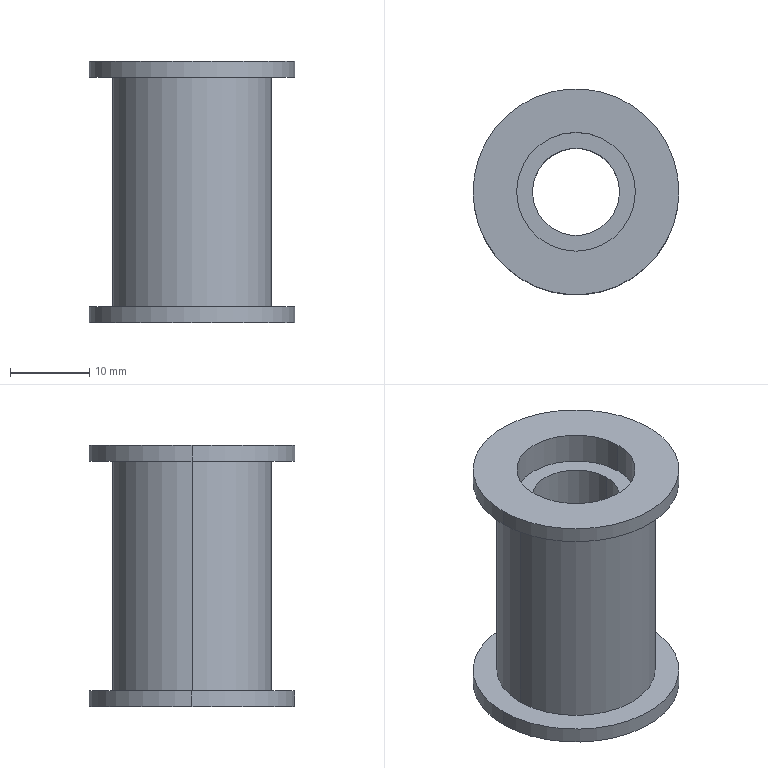Part | STEP file | (PA01.001.LX017) Idler C | 1 solid | 18 faces | box 26 x 26 x 33 mm | volume 7445 mm3 | cylinder 12 | plane 6 | commonest cylinder face diameters 15 x4 26 x4 11 x2 20 x2
STEP:
#1=CARTESIAN_POINT('',(0.,0.,0.));
#2=DIRECTION('',(0.,0.,1.));
#3=DIRECTION('',(1.,0.,0.));
#4=AXIS2_PLACEMENT_3D('',#1,#2,#3);
#5=CARTESIAN_POINT('',(-7.5,0.,-12.5));
#6=VERTEX_POINT('',#5);
#7=CARTESIAN_POINT('',(-7.5,0.,-16.5));
#8=VERTEX_POINT('',#7);
#9=CARTESIAN_POINT('',(-7.5,0.,-12.5));
#10=DIRECTION('',(0.,0.,-1.));
#11=VECTOR('',#10,1.);
#12=LINE('',#9,#11);
#13=CARTESIAN_POINT('',(0.,0.,-12.5));
#14=DIRECTION('',(0.,0.,-1.));
#15=DIRECTION('',(-1.,0.,0.));
#16=AXIS2_PLACEMENT_3D('',#13,#14,#15);
#17=CYLINDRICAL_SURFACE('',#16,7.5);
#18=CARTESIAN_POINT('',(6.283,0.));
#19=DIRECTION('',(0.,1.));
#20=VECTOR('',#19,1.);
#21=LINE('',#18,#20);
#22=(GEOMETRIC_REPRESENTATION_CONTEXT(2)PARAMETRIC_REPRESENTATION_CONTEXT()REPRESENTATION_CONTEXT('',''));
#23=DEFINITIONAL_REPRESENTATION('',(#21),#22);
#24=PCURVE('',#17,#23);
#25=CARTESIAN_POINT('',(0.,0.,-12.5));
#26=DIRECTION('',(0.,0.,-1.));
#27=DIRECTION('',(-1.,0.,0.));
#28=AXIS2_PLACEMENT_3D('',#25,#26,#27);
#29=CYLINDRICAL_SURFACE('',#28,7.5);
#30=CARTESIAN_POINT('',(0.,0.));
#31=DIRECTION('',(0.,1.));
#32=VECTOR('',#31,1.);
#33=LINE('',#30,#32);
#34=(GEOMETRIC_REPRESENTATION_CONTEXT(2)PARAMETRIC_REPRESENTATION_CONTEXT()REPRESENTATION_CONTEXT('',''));
#35=DEFINITIONAL_REPRESENTATION('',(#33),#34);
#36=PCURVE('',#29,#35);
#37=SURFACE_CURVE('',#12,(#24,#36),.PCURVE_S1.);
#38=EDGE_CURVE('',#6,#8,#37,.T.);
#39=ORIENTED_EDGE('',*,*,#38,.T.);
#40=CARTESIAN_POINT('',(7.5,0.,-16.5));
#41=VERTEX_POINT('',#40);
#42=CARTESIAN_POINT('',(0.,0.,-16.5));
#43=DIRECTION('',(0.,0.,-1.));
#44=DIRECTION('',(-1.,0.,0.));
#45=AXIS2_PLACEMENT_3D('',#42,#43,#44);
#46=CIRCLE('',#45,7.5);
#47=CARTESIAN_POINT('',(0.,4.));
#48=DIRECTION('',(1.,0.));
#49=VECTOR('',#48,1.);
#50=LINE('',#47,#49);
#51=(GEOMETRIC_REPRESENTATION_CONTEXT(2)PARAMETRIC_REPRESENTATION_CONTEXT()REPRESENTATION_CONTEXT('',''));
#52=DEFINITIONAL_REPRESENTATION('',(#50),#51);
#53=PCURVE('',#17,#52);
#54=CARTESIAN_POINT('',(0.,0.,-16.5));
#55=DIRECTION('',(0.,0.,-1.));
#56=DIRECTION('',(-1.,0.,0.));
#57=AXIS2_PLACEMENT_3D('',#54,#55,#56);
#58=PLANE('',#57);
#59=CARTESIAN_POINT('',(0.,0.));
#60=DIRECTION('',(1.,0.));
#61=AXIS2_PLACEMENT_2D('',#59,#60);
#62=CIRCLE('',#61,7.5);
#63=(GEOMETRIC_REPRESENTATION_CONTEXT(2)PARAMETRIC_REPRESENTATION_CONTEXT()REPRESENTATION_CONTEXT('',''));
#64=DEFINITIONAL_REPRESENTATION('',(#62),#63);
#65=PCURVE('',#58,#64);
#66=SURFACE_CURVE('',#46,(#53,#65),.PCURVE_S1.);
#67=EDGE_CURVE('',#41,#8,#66,.T.);
#68=ORIENTED_EDGE('',*,*,#67,.F.);
#69=CARTESIAN_POINT('',(7.5,0.,-12.5));
#70=VERTEX_POINT('',#69);
#71=CARTESIAN_POINT('',(7.5,0.,-12.5));
#72=DIRECTION('',(0.,0.,-1.));
#73=VECTOR('',#72,1.);
#74=LINE('',#71,#73);
#75=CARTESIAN_POINT('',(3.142,0.));
#76=DIRECTION('',(0.,1.));
#77=VECTOR('',#76,1.);
#78=LINE('',#75,#77);
#79=(GEOMETRIC_REPRESENTATION_CONTEXT(2)PARAMETRIC_REPRESENTATION_CONTEXT()REPRESENTATION_CONTEXT('',''));
#80=DEFINITIONAL_REPRESENTATION('',(#78),#79);
#81=PCURVE('',#17,#80);
#82=CARTESIAN_POINT('',(3.142,0.));
#83=DIRECTION('',(0.,1.));
#84=VECTOR('',#83,1.);
#85=LINE('',#82,#84);
#86=(GEOMETRIC_REPRESENTATION_CONTEXT(2)PARAMETRIC_REPRESENTATION_CONTEXT()REPRESENTATION_CONTEXT('',''));
#87=DEFINITIONAL_REPRESENTATION('',(#85),#86);
#88=PCURVE('',#29,#87);
#89=SURFACE_CURVE('',#74,(#81,#88),.PCURVE_S1.);
#90=EDGE_CURVE('',#70,#41,#89,.T.);
#91=ORIENTED_EDGE('',*,*,#90,.F.);
#92=CARTESIAN_POINT('',(0.,0.,-12.5));
#93=DIRECTION('',(0.,0.,-1.));
#94=DIRECTION('',(-1.,0.,0.));
#95=AXIS2_PLACEMENT_3D('',#92,#93,#94);
#96=CIRCLE('',#95,7.5);
#97=CARTESIAN_POINT('',(0.,0.));
#98=DIRECTION('',(1.,0.));
#99=VECTOR('',#98,1.);
#100=LINE('',#97,#99);
#101=(GEOMETRIC_REPRESENTATION_CONTEXT(2)PARAMETRIC_REPRESENTATION_CONTEXT()REPRESENTATION_CONTEXT('',''));
#102=DEFINITIONAL_REPRESENTATION('',(#100),#101);
#103=PCURVE('',#17,#102);
#104=CARTESIAN_POINT('',(0.,0.,-12.5));
#105=DIRECTION('',(0.,0.,-1.));
#106=DIRECTION('',(-1.,0.,0.));
#107=AXIS2_PLACEMENT_3D('',#104,#105,#106);
#108=PLANE('',#107);
#109=CARTESIAN_POINT('',(0.,0.));
#110=DIRECTION('',(1.,0.));
#111=AXIS2_PLACEMENT_2D('',#109,#110);
#112=CIRCLE('',#111,7.5);
#113=(GEOMETRIC_REPRESENTATION_CONTEXT(2)PARAMETRIC_REPRESENTATION_CONTEXT()REPRESENTATION_CONTEXT('',''));
#114=DEFINITIONAL_REPRESENTATION('',(#112),#113);
#115=PCURVE('',#108,#114);
#116=SURFACE_CURVE('',#96,(#103,#115),.PCURVE_S1.);
#117=EDGE_CURVE('',#70,#6,#116,.T.);
#118=ORIENTED_EDGE('',*,*,#117,.T.);
#119=EDGE_LOOP('',(#39,#68,#91,#118));
#120=FACE_BOUND('',#119,.F.);
#121=ADVANCED_FACE('',(#120),#17,.F.);
#122=CARTESIAN_POINT('',(7.5,0.,12.5));
#123=VERTEX_POINT('',#122);
#124=CARTESIAN_POINT('',(7.5,0.,16.5));
#125=VERTEX_POINT('',#124);
#126=CARTESIAN_POINT('',(7.5,0.,12.5));
#127=DIRECTION('',(0.,0.,1.));
#128=VECTOR('',#127,1.);
#129=LINE('',#126,#128);
#130=CARTESIAN_POINT('',(0.,0.,12.5));
#131=DIRECTION('',(0.,0.,1.));
#132=DIRECTION('',(1.,0.,0.));
#133=AXIS2_PLACEMENT_3D('',#130,#131,#132);
#134=CYLINDRICAL_SURFACE('',#133,7.5);
#135=CARTESIAN_POINT('',(6.283,0.));
#136=DIRECTION('',(0.,1.));
#137=VECTOR('',#136,1.);
#138=LINE('',#135,#137);
#139=(GEOMETRIC_REPRESENTATION_CONTEXT(2)PARAMETRIC_REPRESENTATION_CONTEXT()REPRESENTATION_CONTEXT('',''));
#140=DEFINITIONAL_REPRESENTATION('',(#138),#139);
#141=PCURVE('',#134,#140);
#142=CARTESIAN_POINT('',(0.,0.,12.5));
#143=DIRECTION('',(0.,0.,1.));
#144=DIRECTION('',(1.,0.,0.));
#145=AXIS2_PLACEMENT_3D('',#142,#143,#144);
#146=CYLINDRICAL_SURFACE('',#145,7.5);
#147=CARTESIAN_POINT('',(0.,0.));
#148=DIRECTION('',(0.,1.));
#149=VECTOR('',#148,1.);
#150=LINE('',#147,#149);
#151=(GEOMETRIC_REPRESENTATION_CONTEXT(2)PARAMETRIC_REPRESENTATION_CONTEXT()REPRESENTATION_CONTEXT('',''));
#152=DEFINITIONAL_REPRESENTATION('',(#150),#151);
#153=PCURVE('',#146,#152);
#154=SURFACE_CURVE('',#129,(#141,#153),.PCURVE_S1.);
#155=EDGE_CURVE('',#123,#125,#154,.T.);
#156=ORIENTED_EDGE('',*,*,#155,.T.);
#157=CARTESIAN_POINT('',(-7.5,0.,16.5));
#158=VERTEX_POINT('',#157);
#159=CARTESIAN_POINT('',(0.,0.,16.5));
#160=DIRECTION('',(0.,0.,1.));
#161=DIRECTION('',(1.,0.,0.));
#162=AXIS2_PLACEMENT_3D('',#159,#160,#161);
#163=CIRCLE('',#162,7.5);
#164=CARTESIAN_POINT('',(0.,4.));
#165=DIRECTION('',(1.,0.));
#166=VECTOR('',#165,1.);
#167=LINE('',#164,#166);
#168=(GEOMETRIC_REPRESENTATION_CONTEXT(2)PARAMETRIC_REPRESENTATION_CONTEXT()REPRESENTATION_CONTEXT('',''));
#169=DEFINITIONAL_REPRESENTATION('',(#167),#168);
#170=PCURVE('',#134,#169);
#171=CARTESIAN_POINT('',(0.,0.,16.5));
#172=DIRECTION('',(0.,0.,1.));
#173=DIRECTION('',(1.,0.,0.));
#174=AXIS2_PLACEMENT_3D('',#171,#172,#173);
#175=PLANE('',#174);
#176=CARTESIAN_POINT('',(0.,0.));
#177=DIRECTION('',(1.,0.));
#178=AXIS2_PLACEMENT_2D('',#176,#177);
#179=CIRCLE('',#178,7.5);
#180=(GEOMETRIC_REPRESENTATION_CONTEXT(2)PARAMETRIC_REPRESENTATION_CONTEXT()REPRESENTATION_CONTEXT('',''));
#181=DEFINITIONAL_REPRESENTATION('',(#179),#180);
#182=PCURVE('',#175,#181);
#183=SURFACE_CURVE('',#163,(#170,#182),.PCURVE_S1.);
#184=EDGE_CURVE('',#158,#125,#183,.T.);
#185=ORIENTED_EDGE('',*,*,#184,.F.);
#186=CARTESIAN_POINT('',(-7.5,0.,12.5));
#187=VERTEX_POINT('',#186);
#188=CARTESIAN_POINT('',(-7.5,0.,12.5));
#189=DIRECTION('',(0.,0.,1.));
#190=VECTOR('',#189,1.);
#191=LINE('',#188,#190);
#192=CARTESIAN_POINT('',(3.142,0.));
#193=DIRECTION('',(0.,1.));
#194=VECTOR('',#193,1.);
#195=LINE('',#192,#194);
#196=(GEOMETRIC_REPRESENTATION_CONTEXT(2)PARAMETRIC_REPRESENTATION_CONTEXT()REPRESENTATION_CONTEXT('',''));
#197=DEFINITIONAL_REPRESENTATION('',(#195),#196);
#198=PCURVE('',#134,#197);
#199=CARTESIAN_POINT('',(3.142,0.));
#200=DIRECTION('',(0.,1.));
#201=VECTOR('',#200,1.);
#202=LINE('',#199,#201);
#203=(GEOMETRIC_REPRESENTATION_CONTEXT(2)PARAMETRIC_REPRESENTATION_CONTEXT()REPRESENTATION_CONTEXT('',''));
#204=DEFINITIONAL_REPRESENTATION('',(#202),#203);
#205=PCURVE('',#146,#204);
#206=SURFACE_CURVE('',#191,(#198,#205),.PCURVE_S1.);
#207=EDGE_CURVE('',#187,#158,#206,.T.);
#208=ORIENTED_EDGE('',*,*,#207,.F.);
#209=CARTESIAN_POINT('',(0.,0.,12.5));
#210=DIRECTION('',(0.,0.,1.));
#211=DIRECTION('',(1.,0.,0.));
#212=AXIS2_PLACEMENT_3D('',#209,#210,#211);
#213=CIRCLE('',#212,7.5);
#214=CARTESIAN_POINT('',(0.,0.));
#215=DIRECTION('',(1.,0.));
#216=VECTOR('',#215,1.);
#217=LINE('',#214,#216);
#218=(GEOMETRIC_REPRESENTATION_CONTEXT(2)PARAMETRIC_REPRESENTATION_CONTEXT()REPRESENTATION_CONTEXT('',''));
#219=DEFINITIONAL_REPRESENTATION('',(#217),#218);
#220=PCURVE('',#134,#219);
#221=CARTESIAN_POINT('',(0.,0.,12.5));
#222=DIRECTION('',(0.,0.,1.));
#223=DIRECTION('',(1.,0.,0.));
#224=AXIS2_PLACEMENT_3D('',#221,#222,#223);
#225=PLANE('',#224);
#226=CARTESIAN_POINT('',(0.,0.));
#227=DIRECTION('',(1.,0.));
#228=AXIS2_PLACEMENT_2D('',#226,#227);
#229=CIRCLE('',#228,7.5);
#230=(GEOMETRIC_REPRESENTATION_CONTEXT(2)PARAMETRIC_REPRESENTATION_CONTEXT()REPRESENTATION_CONTEXT('',''));
#231=DEFINITIONAL_REPRESENTATION('',(#229),#230);
#232=PCURVE('',#225,#231);
#233=SURFACE_CURVE('',#213,(#220,#232),.PCURVE_S1.);
#234=EDGE_CURVE('',#187,#123,#233,.T.);
#235=ORIENTED_EDGE('',*,*,#234,.T.);
#236=EDGE_LOOP('',(#156,#185,#208,#235));
#237=FACE_BOUND('',#236,.F.);
#238=ADVANCED_FACE('',(#237),#134,.F.);
#239=CARTESIAN_POINT('',(-13.,0.,-16.5));
#240=VERTEX_POINT('',#239);
#241=CARTESIAN_POINT('',(13.,0.,-16.5));
#242=VERTEX_POINT('',#241);
#243=CARTESIAN_POINT('',(0.,0.,-16.5));
#244=DIRECTION('',(0.,0.,-1.));
#245=DIRECTION('',(-1.,0.,0.));
#246=AXIS2_PLACEMENT_3D('',#243,#244,#245);
#247=CIRCLE('',#246,13.);
#248=CARTESIAN_POINT('',(0.,0.,-16.5));
#249=DIRECTION('',(0.,0.,1.));
#250=DIRECTION('',(1.,0.,0.));
#251=AXIS2_PLACEMENT_3D('',#248,#249,#250);
#252=CYLINDRICAL_SURFACE('',#251,13.);
#253=CARTESIAN_POINT('',(3.142,0.));
#254=DIRECTION('',(-1.,0.));
#255=VECTOR('',#254,1.);
#256=LINE('',#253,#255);
#257=(GEOMETRIC_REPRESENTATION_CONTEXT(2)PARAMETRIC_REPRESENTATION_CONTEXT()REPRESENTATION_CONTEXT('',''));
#258=DEFINITIONAL_REPRESENTATION('',(#256),#257);
#259=PCURVE('',#252,#258);
#260=CARTESIAN_POINT('',(0.,0.));
#261=DIRECTION('',(1.,0.));
#262=AXIS2_PLACEMENT_2D('',#260,#261);
#263=CIRCLE('',#262,13.);
#264=(GEOMETRIC_REPRESENTATION_CONTEXT(2)PARAMETRIC_REPRESENTATION_CONTEXT()REPRESENTATION_CONTEXT('',''));
#265=DEFINITIONAL_REPRESENTATION('',(#263),#264);
#266=PCURVE('',#58,#265);
#267=SURFACE_CURVE('',#247,(#259,#266),.PCURVE_S1.);
#268=EDGE_CURVE('',#240,#242,#267,.T.);
#269=ORIENTED_EDGE('',*,*,#268,.F.);
#270=CARTESIAN_POINT('',(-13.,0.,-14.5));
#271=VERTEX_POINT('',#270);
#272=CARTESIAN_POINT('',(-13.,0.,-16.5));
#273=DIRECTION('',(0.,0.,1.));
#274=VECTOR('',#273,1.);
#275=LINE('',#272,#274);
#276=CARTESIAN_POINT('',(3.142,0.));
#277=DIRECTION('',(0.,1.));
#278=VECTOR('',#277,1.);
#279=LINE('',#276,#278);
#280=(GEOMETRIC_REPRESENTATION_CONTEXT(2)PARAMETRIC_REPRESENTATION_CONTEXT()REPRESENTATION_CONTEXT('',''));
#281=DEFINITIONAL_REPRESENTATION('',(#279),#280);
#282=PCURVE('',#252,#281);
#283=CARTESIAN_POINT('',(0.,0.,-16.5));
#284=DIRECTION('',(0.,0.,1.));
#285=DIRECTION('',(1.,0.,0.));
#286=AXIS2_PLACEMENT_3D('',#283,#284,#285);
#287=CYLINDRICAL_SURFACE('',#286,13.);
#288=CARTESIAN_POINT('',(3.142,0.));
#289=DIRECTION('',(0.,1.));
#290=VECTOR('',#289,1.);
#291=LINE('',#288,#290);
#292=(GEOMETRIC_REPRESENTATION_CONTEXT(2)PARAMETRIC_REPRESENTATION_CONTEXT()REPRESENTATION_CONTEXT('',''));
#293=DEFINITIONAL_REPRESENTATION('',(#291),#292);
#294=PCURVE('',#287,#293);
#295=SURFACE_CURVE('',#275,(#282,#294),.PCURVE_S1.);
#296=EDGE_CURVE('',#240,#271,#295,.T.);
#297=ORIENTED_EDGE('',*,*,#296,.T.);
#298=CARTESIAN_POINT('',(13.,0.,-14.5));
#299=VERTEX_POINT('',#298);
#300=CARTESIAN_POINT('',(0.,0.,-14.5));
#301=DIRECTION('',(0.,0.,-1.));
#302=DIRECTION('',(-1.,0.,0.));
#303=AXIS2_PLACEMENT_3D('',#300,#301,#302);
#304=CIRCLE('',#303,13.);
#305=CARTESIAN_POINT('',(3.142,2.));
#306=DIRECTION('',(-1.,0.));
#307=VECTOR('',#306,1.);
#308=LINE('',#305,#307);
#309=(GEOMETRIC_REPRESENTATION_CONTEXT(2)PARAMETRIC_REPRESENTATION_CONTEXT()REPRESENTATION_CONTEXT('',''));
#310=DEFINITIONAL_REPRESENTATION('',(#308),#309);
#311=PCURVE('',#252,#310);
#312=CARTESIAN_POINT('',(0.,0.,-14.5));
#313=DIRECTION('',(0.,0.,-1.));
#314=DIRECTION('',(-1.,0.,0.));
#315=AXIS2_PLACEMENT_3D('',#312,#313,#314);
#316=PLANE('',#315);
#317=CARTESIAN_POINT('',(0.,0.));
#318=DIRECTION('',(1.,0.));
#319=AXIS2_PLACEMENT_2D('',#317,#318);
#320=CIRCLE('',#319,13.);
#321=(GEOMETRIC_REPRESENTATION_CONTEXT(2)PARAMETRIC_REPRESENTATION_CONTEXT()REPRESENTATION_CONTEXT('',''));
#322=DEFINITIONAL_REPRESENTATION('',(#320),#321);
#323=PCURVE('',#316,#322);
#324=SURFACE_CURVE('',#304,(#311,#323),.PCURVE_S1.);
#325=EDGE_CURVE('',#271,#299,#324,.T.);
#326=ORIENTED_EDGE('',*,*,#325,.T.);
#327=CARTESIAN_POINT('',(13.,0.,-16.5));
#328=DIRECTION('',(0.,0.,1.));
#329=VECTOR('',#328,1.);
#330=LINE('',#327,#329);
#331=CARTESIAN_POINT('',(0.,0.));
#332=DIRECTION('',(0.,1.));
#333=VECTOR('',#332,1.);
#334=LINE('',#331,#333);
#335=(GEOMETRIC_REPRESENTATION_CONTEXT(2)PARAMETRIC_REPRESENTATION_CONTEXT()REPRESENTATION_CONTEXT('',''));
#336=DEFINITIONAL_REPRESENTATION('',(#334),#335);
#337=PCURVE('',#252,#336);
#338=CARTESIAN_POINT('',(6.283,0.));
#339=DIRECTION('',(0.,1.));
#340=VECTOR('',#339,1.);
#341=LINE('',#338,#340);
#342=(GEOMETRIC_REPRESENTATION_CONTEXT(2)PARAMETRIC_REPRESENTATION_CONTEXT()REPRESENTATION_CONTEXT('',''));
#343=DEFINITIONAL_REPRESENTATION('',(#341),#342);
#344=PCURVE('',#287,#343);
#345=SURFACE_CURVE('',#330,(#337,#344),.PCURVE_S1.);
#346=EDGE_CURVE('',#242,#299,#345,.T.);
#347=ORIENTED_EDGE('',*,*,#346,.F.);
#348=EDGE_LOOP('',(#269,#297,#326,#347));
#349=FACE_BOUND('',#348,.T.);
#350=ADVANCED_FACE('',(#349),#252,.T.);
#351=CARTESIAN_POINT('',(13.,0.,16.5));
#352=VERTEX_POINT('',#351);
#353=CARTESIAN_POINT('',(-13.,0.,16.5));
#354=VERTEX_POINT('',#353);
#355=CARTESIAN_POINT('',(0.,0.,16.5));
#356=DIRECTION('',(0.,0.,1.));
#357=DIRECTION('',(1.,0.,0.));
#358=AXIS2_PLACEMENT_3D('',#355,#356,#357);
#359=CIRCLE('',#358,13.);
#360=CARTESIAN_POINT('',(0.,0.,16.5));
#361=DIRECTION('',(0.,0.,-1.));
#362=DIRECTION('',(-1.,0.,0.));
#363=AXIS2_PLACEMENT_3D('',#360,#361,#362);
#364=CYLINDRICAL_SURFACE('',#363,13.);
#365=CARTESIAN_POINT('',(3.142,0.));
#366=DIRECTION('',(-1.,0.));
#367=VECTOR('',#366,1.);
#368=LINE('',#365,#367);
#369=(GEOMETRIC_REPRESENTATION_CONTEXT(2)PARAMETRIC_REPRESENTATION_CONTEXT()REPRESENTATION_CONTEXT('',''));
#370=DEFINITIONAL_REPRESENTATION('',(#368),#369);
#371=PCURVE('',#364,#370);
#372=CARTESIAN_POINT('',(0.,0.));
#373=DIRECTION('',(1.,0.));
#374=AXIS2_PLACEMENT_2D('',#372,#373);
#375=CIRCLE('',#374,13.);
#376=(GEOMETRIC_REPRESENTATION_CONTEXT(2)PARAMETRIC_REPRESENTATION_CONTEXT()REPRESENTATION_CONTEXT('',''));
#377=DEFINITIONAL_REPRESENTATION('',(#375),#376);
#378=PCURVE('',#175,#377);
#379=SURFACE_CURVE('',#359,(#371,#378),.PCURVE_S1.);
#380=EDGE_CURVE('',#352,#354,#379,.T.);
#381=ORIENTED_EDGE('',*,*,#380,.F.);
#382=CARTESIAN_POINT('',(13.,0.,14.5));
#383=VERTEX_POINT('',#382);
#384=CARTESIAN_POINT('',(13.,0.,16.5));
#385=DIRECTION('',(0.,0.,-1.));
#386=VECTOR('',#385,1.);
#387=LINE('',#384,#386);
#388=CARTESIAN_POINT('',(3.142,0.));
#389=DIRECTION('',(0.,1.));
#390=VECTOR('',#389,1.);
#391=LINE('',#388,#390);
#392=(GEOMETRIC_REPRESENTATION_CONTEXT(2)PARAMETRIC_REPRESENTATION_CONTEXT()REPRESENTATION_CONTEXT('',''));
#393=DEFINITIONAL_REPRESENTATION('',(#391),#392);
#394=PCURVE('',#364,#393);
#395=CARTESIAN_POINT('',(0.,0.,16.5));
#396=DIRECTION('',(0.,0.,-1.));
#397=DIRECTION('',(-1.,0.,0.));
#398=AXIS2_PLACEMENT_3D('',#395,#396,#397);
#399=CYLINDRICAL_SURFACE('',#398,13.);
#400=CARTESIAN_POINT('',(3.142,0.));
#401=DIRECTION('',(0.,1.));
#402=VECTOR('',#401,1.);
#403=LINE('',#400,#402);
#404=(GEOMETRIC_REPRESENTATION_CONTEXT(2)PARAMETRIC_REPRESENTATION_CONTEXT()REPRESENTATION_CONTEXT('',''));
#405=DEFINITIONAL_REPRESENTATION('',(#403),#404);
#406=PCURVE('',#399,#405);
#407=SURFACE_CURVE('',#387,(#394,#406),.PCURVE_S1.);
#408=EDGE_CURVE('',#352,#383,#407,.T.);
#409=ORIENTED_EDGE('',*,*,#408,.T.);
#410=CARTESIAN_POINT('',(-13.,0.,14.5));
#411=VERTEX_POINT('',#410);
#412=CARTESIAN_POINT('',(0.,0.,14.5));
#413=DIRECTION('',(0.,0.,1.));
#414=DIRECTION('',(1.,0.,0.));
#415=AXIS2_PLACEMENT_3D('',#412,#413,#414);
#416=CIRCLE('',#415,13.);
#417=CARTESIAN_POINT('',(3.142,2.));
#418=DIRECTION('',(-1.,0.));
#419=VECTOR('',#418,1.);
#420=LINE('',#417,#419);
#421=(GEOMETRIC_REPRESENTATION_CONTEXT(2)PARAMETRIC_REPRESENTATION_CONTEXT()REPRESENTATION_CONTEXT('',''));
#422=DEFINITIONAL_REPRESENTATION('',(#420),#421);
#423=PCURVE('',#364,#422);
#424=CARTESIAN_POINT('',(0.,0.,14.5));
#425=DIRECTION('',(0.,0.,1.));
#426=DIRECTION('',(1.,0.,0.));
#427=AXIS2_PLACEMENT_3D('',#424,#425,#426);
#428=PLANE('',#427);
#429=CARTESIAN_POINT('',(0.,0.));
#430=DIRECTION('',(1.,0.));
#431=AXIS2_PLACEMENT_2D('',#429,#430);
#432=CIRCLE('',#431,13.);
#433=(GEOMETRIC_REPRESENTATION_CONTEXT(2)PARAMETRIC_REPRESENTATION_CONTEXT()REPRESENTATION_CONTEXT('',''));
#434=DEFINITIONAL_REPRESENTATION('',(#432),#433);
#435=PCURVE('',#428,#434);
#436=SURFACE_CURVE('',#416,(#423,#435),.PCURVE_S1.);
#437=EDGE_CURVE('',#383,#411,#436,.T.);
#438=ORIENTED_EDGE('',*,*,#437,.T.);
#439=CARTESIAN_POINT('',(-13.,0.,16.5));
#440=DIRECTION('',(0.,0.,-1.));
#441=VECTOR('',#440,1.);
#442=LINE('',#439,#441);
#443=CARTESIAN_POINT('',(0.,0.));
#444=DIRECTION('',(0.,1.));
#445=VECTOR('',#444,1.);
#446=LINE('',#443,#445);
#447=(GEOMETRIC_REPRESENTATION_CONTEXT(2)PARAMETRIC_REPRESENTATION_CONTEXT()REPRESENTATION_CONTEXT('',''));
#448=DEFINITIONAL_REPRESENTATION('',(#446),#447);
#449=PCURVE('',#364,#448);
#450=CARTESIAN_POINT('',(6.283,0.));
#451=DIRECTION('',(0.,1.));
#452=VECTOR('',#451,1.);
#453=LINE('',#450,#452);
#454=(GEOMETRIC_REPRESENTATION_CONTEXT(2)PARAMETRIC_REPRESENTATION_CONTEXT()REPRESENTATION_CONTEXT('',''));
#455=DEFINITIONAL_REPRESENTATION('',(#453),#454);
#456=PCURVE('',#399,#455);
#457=SURFACE_CURVE('',#442,(#449,#456),.PCURVE_S1.);
#458=EDGE_CURVE('',#354,#411,#457,.T.);
#459=ORIENTED_EDGE('',*,*,#458,.F.);
#460=EDGE_LOOP('',(#381,#409,#438,#459));
#461=FACE_BOUND('',#460,.T.);
#462=ADVANCED_FACE('',(#461),#364,.T.);
#463=CARTESIAN_POINT('',(10.,0.,14.5));
#464=VERTEX_POINT('',#463);
#465=CARTESIAN_POINT('',(-10.,0.,14.5));
#466=VERTEX_POINT('',#465);
#467=CARTESIAN_POINT('',(0.,0.,14.5));
#468=DIRECTION('',(0.,0.,1.));
#469=DIRECTION('',(1.,0.,0.));
#470=AXIS2_PLACEMENT_3D('',#467,#468,#469);
#471=CIRCLE('',#470,10.);
#472=CARTESIAN_POINT('',(0.,0.,14.5));
#473=DIRECTION('',(0.,0.,-1.));
#474=DIRECTION('',(-1.,0.,0.));
#475=AXIS2_PLACEMENT_3D('',#472,#473,#474);
#476=CYLINDRICAL_SURFACE('',#475,10.);
#477=CARTESIAN_POINT('',(3.142,0.));
#478=DIRECTION('',(-1.,0.));
#479=VECTOR('',#478,1.);
#480=LINE('',#477,#479);
#481=(GEOMETRIC_REPRESENTATION_CONTEXT(2)PARAMETRIC_REPRESENTATION_CONTEXT()REPRESENTATION_CONTEXT('',''));
#482=DEFINITIONAL_REPRESENTATION('',(#480),#481);
#483=PCURVE('',#476,#482);
#484=CARTESIAN_POINT('',(0.,0.));
#485=DIRECTION('',(1.,0.));
#486=AXIS2_PLACEMENT_2D('',#484,#485);
#487=CIRCLE('',#486,10.);
#488=(GEOMETRIC_REPRESENTATION_CONTEXT(2)PARAMETRIC_REPRESENTATION_CONTEXT()REPRESENTATION_CONTEXT('',''));
#489=DEFINITIONAL_REPRESENTATION('',(#487),#488);
#490=PCURVE('',#428,#489);
#491=SURFACE_CURVE('',#471,(#483,#490),.PCURVE_S1.);
#492=EDGE_CURVE('',#464,#466,#491,.T.);
#493=ORIENTED_EDGE('',*,*,#492,.F.);
#494=CARTESIAN_POINT('',(10.,0.,-14.5));
#495=VERTEX_POINT('',#494);
#496=CARTESIAN_POINT('',(10.,0.,14.5));
#497=DIRECTION('',(0.,0.,-1.));
#498=VECTOR('',#497,1.);
#499=LINE('',#496,#498);
#500=CARTESIAN_POINT('',(3.142,0.));
#501=DIRECTION('',(0.,1.));
#502=VECTOR('',#501,1.);
#503=LINE('',#500,#502);
#504=(GEOMETRIC_REPRESENTATION_CONTEXT(2)PARAMETRIC_REPRESENTATION_CONTEXT()REPRESENTATION_CONTEXT('',''));
#505=DEFINITIONAL_REPRESENTATION('',(#503),#504);
#506=PCURVE('',#476,#505);
#507=CARTESIAN_POINT('',(0.,0.,14.5));
#508=DIRECTION('',(0.,0.,-1.));
#509=DIRECTION('',(-1.,0.,0.));
#510=AXIS2_PLACEMENT_3D('',#507,#508,#509);
#511=CYLINDRICAL_SURFACE('',#510,10.);
#512=CARTESIAN_POINT('',(3.142,0.));
#513=DIRECTION('',(0.,1.));
#514=VECTOR('',#513,1.);
#515=LINE('',#512,#514);
#516=(GEOMETRIC_REPRESENTATION_CONTEXT(2)PARAMETRIC_REPRESENTATION_CONTEXT()REPRESENTATION_CONTEXT('',''));
#517=DEFINITIONAL_REPRESENTATION('',(#515),#516);
#518=PCURVE('',#511,#517);
#519=SURFACE_CURVE('',#499,(#506,#518),.PCURVE_S1.);
#520=EDGE_CURVE('',#464,#495,#519,.T.);
#521=ORIENTED_EDGE('',*,*,#520,.T.);
#522=CARTESIAN_POINT('',(-10.,0.,-14.5));
#523=VERTEX_POINT('',#522);
#524=CARTESIAN_POINT('',(0.,0.,-14.5));
#525=DIRECTION('',(0.,0.,-1.));
#526=DIRECTION('',(-1.,0.,0.));
#527=AXIS2_PLACEMENT_3D('',#524,#525,#526);
#528=CIRCLE('',#527,10.);
#529=CARTESIAN_POINT('',(0.,29.));
#530=DIRECTION('',(1.,0.));
#531=VECTOR('',#530,1.);
#532=LINE('',#529,#531);
#533=(GEOMETRIC_REPRESENTATION_CONTEXT(2)PARAMETRIC_REPRESENTATION_CONTEXT()REPRESENTATION_CONTEXT('',''));
#534=DEFINITIONAL_REPRESENTATION('',(#532),#533);
#535=PCURVE('',#476,#534);
#536=CARTESIAN_POINT('',(0.,0.));
#537=DIRECTION('',(1.,0.));
#538=AXIS2_PLACEMENT_2D('',#536,#537);
#539=CIRCLE('',#538,10.);
#540=(GEOMETRIC_REPRESENTATION_CONTEXT(2)PARAMETRIC_REPRESENTATION_CONTEXT()REPRESENTATION_CONTEXT('',''));
#541=DEFINITIONAL_REPRESENTATION('',(#539),#540);
#542=PCURVE('',#316,#541);
#543=SURFACE_CURVE('',#528,(#535,#542),.PCURVE_S1.);
#544=EDGE_CURVE('',#523,#495,#543,.T.);
#545=ORIENTED_EDGE('',*,*,#544,.F.);
#546=CARTESIAN_POINT('',(-10.,0.,14.5));
#547=DIRECTION('',(0.,0.,-1.));
#548=VECTOR('',#547,1.);
#549=LINE('',#546,#548);
#550=CARTESIAN_POINT('',(0.,0.));
#551=DIRECTION('',(0.,1.));
#552=VECTOR('',#551,1.);
#553=LINE('',#550,#552);
#554=(GEOMETRIC_REPRESENTATION_CONTEXT(2)PARAMETRIC_REPRESENTATION_CONTEXT()REPRESENTATION_CONTEXT('',''));
#555=DEFINITIONAL_REPRESENTATION('',(#553),#554);
#556=PCURVE('',#476,#555);
#557=CARTESIAN_POINT('',(6.283,0.));
#558=DIRECTION('',(0.,1.));
#559=VECTOR('',#558,1.);
#560=LINE('',#557,#559);
#561=(GEOMETRIC_REPRESENTATION_CONTEXT(2)PARAMETRIC_REPRESENTATION_CONTEXT()REPRESENTATION_CONTEXT('',''));
#562=DEFINITIONAL_REPRESENTATION('',(#560),#561);
#563=PCURVE('',#511,#562);
#564=SURFACE_CURVE('',#549,(#556,#563),.PCURVE_S1.);
#565=EDGE_CURVE('',#466,#523,#564,.T.);
#566=ORIENTED_EDGE('',*,*,#565,.F.);
#567=EDGE_LOOP('',(#493,#521,#545,#566));
#568=FACE_BOUND('',#567,.T.);
#569=ADVANCED_FACE('',(#568),#476,.T.);
#570=CARTESIAN_POINT('',(5.5,0.,-12.5));
#571=VERTEX_POINT('',#570);
#572=CARTESIAN_POINT('',(5.5,0.,12.5));
#573=VERTEX_POINT('',#572);
#574=CARTESIAN_POINT('',(5.5,0.,-16.5));
#575=DIRECTION('',(0.,0.,1.));
#576=VECTOR('',#575,1.);
#577=LINE('',#574,#576);
#578=CARTESIAN_POINT('',(0.,0.,-16.5));
#579=DIRECTION('',(0.,0.,1.));
#580=DIRECTION('',(1.,0.,0.));
#581=AXIS2_PLACEMENT_3D('',#578,#579,#580);
#582=CYLINDRICAL_SURFACE('',#581,5.5);
#583=CARTESIAN_POINT('',(6.283,0.));
#584=DIRECTION('',(0.,1.));
#585=VECTOR('',#584,1.);
#586=LINE('',#583,#585);
#587=(GEOMETRIC_REPRESENTATION_CONTEXT(2)PARAMETRIC_REPRESENTATION_CONTEXT()REPRESENTATION_CONTEXT('',''));
#588=DEFINITIONAL_REPRESENTATION('',(#586),#587);
#589=PCURVE('',#582,#588);
#590=CARTESIAN_POINT('',(0.,0.,-16.5));
#591=DIRECTION('',(0.,0.,1.));
#592=DIRECTION('',(1.,0.,0.));
#593=AXIS2_PLACEMENT_3D('',#590,#591,#592);
#594=CYLINDRICAL_SURFACE('',#593,5.5);
#595=CARTESIAN_POINT('',(0.,0.));
#596=DIRECTION('',(0.,1.));
#597=VECTOR('',#596,1.);
#598=LINE('',#595,#597);
#599=(GEOMETRIC_REPRESENTATION_CONTEXT(2)PARAMETRIC_REPRESENTATION_CONTEXT()REPRESENTATION_CONTEXT('',''));
#600=DEFINITIONAL_REPRESENTATION('',(#598),#599);
#601=PCURVE('',#594,#600);
#602=SURFACE_CURVE('',#577,(#589,#601),.PCURVE_S1.);
#603=EDGE_CURVE('',#571,#573,#602,.T.);
#604=ORIENTED_EDGE('',*,*,#603,.T.);
#605=CARTESIAN_POINT('',(-5.5,0.,12.5));
#606=VERTEX_POINT('',#605);
#607=CARTESIAN_POINT('',(0.,0.,12.5));
#608=DIRECTION('',(0.,0.,-1.));
#609=DIRECTION('',(1.,0.,0.));
#610=AXIS2_PLACEMENT_3D('',#607,#608,#609);
#611=CIRCLE('',#610,5.5);
#612=CARTESIAN_POINT('',(6.283,29.));
#613=DIRECTION('',(-1.,0.));
#614=VECTOR('',#613,1.);
#615=LINE('',#612,#614);
#616=(GEOMETRIC_REPRESENTATION_CONTEXT(2)PARAMETRIC_REPRESENTATION_CONTEXT()REPRESENTATION_CONTEXT('',''));
#617=DEFINITIONAL_REPRESENTATION('',(#615),#616);
#618=PCURVE('',#582,#617);
#619=CARTESIAN_POINT('',(5.5,0.));
#620=CARTESIAN_POINT('',(5.5,-9.526));
#621=CARTESIAN_POINT('',(-2.75,-4.763));
#622=CARTESIAN_POINT('',(-11.,0.));
#623=CARTESIAN_POINT('',(-2.75,4.763));
#624=CARTESIAN_POINT('',(5.5,9.526));
#625=CARTESIAN_POINT('',(5.5,0.));
#626=(BOUNDED_CURVE()B_SPLINE_CURVE(2,(#619,#620,#621,#622,#623,#624,#625),.UNSPECIFIED.,.T.,.F.)B_SPLINE_CURVE_WITH_KNOTS((1,2,2,2,2,1),(-2.094,0.,2.094,4.189,6.283,8.378),.UNSPECIFIED.)CURVE()GEOMETRIC_REPRESENTATION_ITEM()RATIONAL_B_SPLINE_CURVE((1.,0.5,1.,0.5,1.,0.5,1.))REPRESENTATION_ITEM(''));
#627=(GEOMETRIC_REPRESENTATION_CONTEXT(2)PARAMETRIC_REPRESENTATION_CONTEXT()REPRESENTATION_CONTEXT('',''));
#628=DEFINITIONAL_REPRESENTATION('',(#626),#627);
#629=PCURVE('',#225,#628);
#630=SURFACE_CURVE('',#611,(#618,#629),.PCURVE_S1.);
#631=EDGE_CURVE('',#573,#606,#630,.T.);
#632=ORIENTED_EDGE('',*,*,#631,.T.);
#633=CARTESIAN_POINT('',(-5.5,0.,-12.5));
#634=VERTEX_POINT('',#633);
#635=CARTESIAN_POINT('',(-5.5,0.,-16.5));
#636=DIRECTION('',(0.,0.,1.));
#637=VECTOR('',#636,1.);
#638=LINE('',#635,#637);
#639=CARTESIAN_POINT('',(3.142,0.));
#640=DIRECTION('',(0.,1.));
#641=VECTOR('',#640,1.);
#642=LINE('',#639,#641);
#643=(GEOMETRIC_REPRESENTATION_CONTEXT(2)PARAMETRIC_REPRESENTATION_CONTEXT()REPRESENTATION_CONTEXT('',''));
#644=DEFINITIONAL_REPRESENTATION('',(#642),#643);
#645=PCURVE('',#582,#644);
#646=CARTESIAN_POINT('',(3.142,0.));
#647=DIRECTION('',(0.,1.));
#648=VECTOR('',#647,1.);
#649=LINE('',#646,#648);
#650=(GEOMETRIC_REPRESENTATION_CONTEXT(2)PARAMETRIC_REPRESENTATION_CONTEXT()REPRESENTATION_CONTEXT('',''));
#651=DEFINITIONAL_REPRESENTATION('',(#649),#650);
#652=PCURVE('',#594,#651);
#653=SURFACE_CURVE('',#638,(#645,#652),.PCURVE_S1.);
#654=EDGE_CURVE('',#634,#606,#653,.T.);
#655=ORIENTED_EDGE('',*,*,#654,.F.);
#656=CARTESIAN_POINT('',(0.,0.,-12.5));
#657=DIRECTION('',(0.,0.,1.));
#658=DIRECTION('',(-1.,0.,0.));
#659=AXIS2_PLACEMENT_3D('',#656,#657,#658);
#660=CIRCLE('',#659,5.5);
#661=CARTESIAN_POINT('',(3.142,4.));
#662=DIRECTION('',(1.,0.));
#663=VECTOR('',#662,1.);
#664=LINE('',#661,#663);
#665=(GEOMETRIC_REPRESENTATION_CONTEXT(2)PARAMETRIC_REPRESENTATION_CONTEXT()REPRESENTATION_CONTEXT('',''));
#666=DEFINITIONAL_REPRESENTATION('',(#664),#665);
#667=PCURVE('',#582,#666);
#668=CARTESIAN_POINT('',(5.5,0.));
#669=CARTESIAN_POINT('',(5.5,-9.526));
#670=CARTESIAN_POINT('',(-2.75,-4.763));
#671=CARTESIAN_POINT('',(-11.,0.));
#672=CARTESIAN_POINT('',(-2.75,4.763));
#673=CARTESIAN_POINT('',(5.5,9.526));
#674=CARTESIAN_POINT('',(5.5,0.));
#675=(BOUNDED_CURVE()B_SPLINE_CURVE(2,(#668,#669,#670,#671,#672,#673,#674),.UNSPECIFIED.,.T.,.F.)B_SPLINE_CURVE_WITH_KNOTS((1,2,2,2,2,1),(-2.094,0.,2.094,4.189,6.283,8.378),.UNSPECIFIED.)CURVE()GEOMETRIC_REPRESENTATION_ITEM()RATIONAL_B_SPLINE_CURVE((1.,0.5,1.,0.5,1.,0.5,1.))REPRESENTATION_ITEM(''));
#676=(GEOMETRIC_REPRESENTATION_CONTEXT(2)PARAMETRIC_REPRESENTATION_CONTEXT()REPRESENTATION_CONTEXT('',''));
#677=DEFINITIONAL_REPRESENTATION('',(#675),#676);
#678=PCURVE('',#108,#677);
#679=SURFACE_CURVE('',#660,(#667,#678),.PCURVE_S1.);
#680=EDGE_CURVE('',#634,#571,#679,.T.);
#681=ORIENTED_EDGE('',*,*,#680,.T.);
#682=EDGE_LOOP('',(#604,#632,#655,#681));
#683=FACE_BOUND('',#682,.F.);
#684=ADVANCED_FACE('',(#683),#582,.F.);
#685=CARTESIAN_POINT('',(0.,0.,12.5));
#686=DIRECTION('',(0.,0.,-1.));
#687=DIRECTION('',(1.,0.,0.));
#688=AXIS2_PLACEMENT_3D('',#685,#686,#687);
#689=CIRCLE('',#688,5.5);
#690=CARTESIAN_POINT('',(6.283,29.));
#691=DIRECTION('',(-1.,0.));
#692=VECTOR('',#691,1.);
#693=LINE('',#690,#692);
#694=(GEOMETRIC_REPRESENTATION_CONTEXT(2)PARAMETRIC_REPRESENTATION_CONTEXT()REPRESENTATION_CONTEXT('',''));
#695=DEFINITIONAL_REPRESENTATION('',(#693),#694);
#696=PCURVE('',#594,#695);
#697=CARTESIAN_POINT('',(5.5,0.));
#698=CARTESIAN_POINT('',(5.5,-9.526));
#699=CARTESIAN_POINT('',(-2.75,-4.763));
#700=CARTESIAN_POINT('',(-11.,0.));
#701=CARTESIAN_POINT('',(-2.75,4.763));
#702=CARTESIAN_POINT('',(5.5,9.526));
#703=CARTESIAN_POINT('',(5.5,0.));
#704=(BOUNDED_CURVE()B_SPLINE_CURVE(2,(#697,#698,#699,#700,#701,#702,#703),.UNSPECIFIED.,.T.,.F.)B_SPLINE_CURVE_WITH_KNOTS((1,2,2,2,2,1),(-2.094,0.,2.094,4.189,6.283,8.378),.UNSPECIFIED.)CURVE()GEOMETRIC_REPRESENTATION_ITEM()RATIONAL_B_SPLINE_CURVE((1.,0.5,1.,0.5,1.,0.5,1.))REPRESENTATION_ITEM(''));
#705=(GEOMETRIC_REPRESENTATION_CONTEXT(2)PARAMETRIC_REPRESENTATION_CONTEXT()REPRESENTATION_CONTEXT('',''));
#706=DEFINITIONAL_REPRESENTATION('',(#704),#705);
#707=PCURVE('',#225,#706);
#708=SURFACE_CURVE('',#689,(#696,#707),.PCURVE_S1.);
#709=EDGE_CURVE('',#606,#573,#708,.T.);
#710=ORIENTED_EDGE('',*,*,#709,.T.);
#711=ORIENTED_EDGE('',*,*,#603,.F.);
#712=CARTESIAN_POINT('',(0.,0.,-12.5));
#713=DIRECTION('',(0.,0.,1.));
#714=DIRECTION('',(-1.,0.,0.));
#715=AXIS2_PLACEMENT_3D('',#712,#713,#714);
#716=CIRCLE('',#715,5.5);
#717=CARTESIAN_POINT('',(-3.142,4.));
#718=DIRECTION('',(1.,0.));
#719=VECTOR('',#718,1.);
#720=LINE('',#717,#719);
#721=(GEOMETRIC_REPRESENTATION_CONTEXT(2)PARAMETRIC_REPRESENTATION_CONTEXT()REPRESENTATION_CONTEXT('',''));
#722=DEFINITIONAL_REPRESENTATION('',(#720),#721);
#723=PCURVE('',#594,#722);
#724=CARTESIAN_POINT('',(5.5,0.));
#725=CARTESIAN_POINT('',(5.5,-9.526));
#726=CARTESIAN_POINT('',(-2.75,-4.763));
#727=CARTESIAN_POINT('',(-11.,0.));
#728=CARTESIAN_POINT('',(-2.75,4.763));
#729=CARTESIAN_POINT('',(5.5,9.526));
#730=CARTESIAN_POINT('',(5.5,0.));
#731=(BOUNDED_CURVE()B_SPLINE_CURVE(2,(#724,#725,#726,#727,#728,#729,#730),.UNSPECIFIED.,.T.,.F.)B_SPLINE_CURVE_WITH_KNOTS((1,2,2,2,2,1),(-2.094,0.,2.094,4.189,6.283,8.378),.UNSPECIFIED.)CURVE()GEOMETRIC_REPRESENTATION_ITEM()RATIONAL_B_SPLINE_CURVE((1.,0.5,1.,0.5,1.,0.5,1.))REPRESENTATION_ITEM(''));
#732=(GEOMETRIC_REPRESENTATION_CONTEXT(2)PARAMETRIC_REPRESENTATION_CONTEXT()REPRESENTATION_CONTEXT('',''));
#733=DEFINITIONAL_REPRESENTATION('',(#731),#732);
#734=PCURVE('',#108,#733);
#735=SURFACE_CURVE('',#716,(#723,#734),.PCURVE_S1.);
#736=EDGE_CURVE('',#571,#634,#735,.T.);
#737=ORIENTED_EDGE('',*,*,#736,.T.);
#738=ORIENTED_EDGE('',*,*,#654,.T.);
#739=EDGE_LOOP('',(#710,#711,#737,#738));
#740=FACE_BOUND('',#739,.F.);
#741=ADVANCED_FACE('',(#740),#594,.F.);
#742=ORIENTED_EDGE('',*,*,#520,.F.);
#743=CARTESIAN_POINT('',(0.,0.,14.5));
#744=DIRECTION('',(0.,0.,1.));
#745=DIRECTION('',(1.,0.,0.));
#746=AXIS2_PLACEMENT_3D('',#743,#744,#745);
#747=CIRCLE('',#746,10.);
#748=CARTESIAN_POINT('',(9.425,0.));
#749=DIRECTION('',(-1.,0.));
#750=VECTOR('',#749,1.);
#751=LINE('',#748,#750);
#752=(GEOMETRIC_REPRESENTATION_CONTEXT(2)PARAMETRIC_REPRESENTATION_CONTEXT()REPRESENTATION_CONTEXT('',''));
#753=DEFINITIONAL_REPRESENTATION('',(#751),#752);
#754=PCURVE('',#511,#753);
#755=CARTESIAN_POINT('',(0.,0.));
#756=DIRECTION('',(1.,0.));
#757=AXIS2_PLACEMENT_2D('',#755,#756);
#758=CIRCLE('',#757,10.);
#759=(GEOMETRIC_REPRESENTATION_CONTEXT(2)PARAMETRIC_REPRESENTATION_CONTEXT()REPRESENTATION_CONTEXT('',''));
#760=DEFINITIONAL_REPRESENTATION('',(#758),#759);
#761=PCURVE('',#428,#760);
#762=SURFACE_CURVE('',#747,(#754,#761),.PCURVE_S1.);
#763=EDGE_CURVE('',#466,#464,#762,.T.);
#764=ORIENTED_EDGE('',*,*,#763,.F.);
#765=ORIENTED_EDGE('',*,*,#565,.T.);
#766=CARTESIAN_POINT('',(0.,0.,-14.5));
#767=DIRECTION('',(0.,0.,-1.));
#768=DIRECTION('',(-1.,0.,0.));
#769=AXIS2_PLACEMENT_3D('',#766,#767,#768);
#770=CIRCLE('',#769,10.);
#771=CARTESIAN_POINT('',(0.,29.));
#772=DIRECTION('',(1.,0.));
#773=VECTOR('',#772,1.);
#774=LINE('',#771,#773);
#775=(GEOMETRIC_REPRESENTATION_CONTEXT(2)PARAMETRIC_REPRESENTATION_CONTEXT()REPRESENTATION_CONTEXT('',''));
#776=DEFINITIONAL_REPRESENTATION('',(#774),#775);
#777=PCURVE('',#511,#776);
#778=CARTESIAN_POINT('',(0.,0.));
#779=DIRECTION('',(1.,0.));
#780=AXIS2_PLACEMENT_2D('',#778,#779);
#781=CIRCLE('',#780,10.);
#782=(GEOMETRIC_REPRESENTATION_CONTEXT(2)PARAMETRIC_REPRESENTATION_CONTEXT()REPRESENTATION_CONTEXT('',''));
#783=DEFINITIONAL_REPRESENTATION('',(#781),#782);
#784=PCURVE('',#316,#783);
#785=SURFACE_CURVE('',#770,(#777,#784),.PCURVE_S1.);
#786=EDGE_CURVE('',#495,#523,#785,.T.);
#787=ORIENTED_EDGE('',*,*,#786,.F.);
#788=EDGE_LOOP('',(#742,#764,#765,#787));
#789=FACE_BOUND('',#788,.T.);
#790=ADVANCED_FACE('',(#789),#511,.T.);
#791=CARTESIAN_POINT('',(0.,0.,14.5));
#792=DIRECTION('',(0.,0.,1.));
#793=DIRECTION('',(1.,0.,0.));
#794=AXIS2_PLACEMENT_3D('',#791,#792,#793);
#795=CIRCLE('',#794,13.);
#796=CARTESIAN_POINT('',(0.,0.));
#797=DIRECTION('',(1.,0.));
#798=AXIS2_PLACEMENT_2D('',#796,#797);
#799=CIRCLE('',#798,13.);
#800=(GEOMETRIC_REPRESENTATION_CONTEXT(2)PARAMETRIC_REPRESENTATION_CONTEXT()REPRESENTATION_CONTEXT('',''));
#801=DEFINITIONAL_REPRESENTATION('',(#799),#800);
#802=PCURVE('',#428,#801);
#803=CARTESIAN_POINT('',(9.425,2.));
#804=DIRECTION('',(-1.,0.));
#805=VECTOR('',#804,1.);
#806=LINE('',#803,#805);
#807=(GEOMETRIC_REPRESENTATION_CONTEXT(2)PARAMETRIC_REPRESENTATION_CONTEXT()REPRESENTATION_CONTEXT('',''));
#808=DEFINITIONAL_REPRESENTATION('',(#806),#807);
#809=PCURVE('',#399,#808);
#810=SURFACE_CURVE('',#795,(#802,#809),.PCURVE_S1.);
#811=EDGE_CURVE('',#411,#383,#810,.T.);
#812=ORIENTED_EDGE('',*,*,#811,.F.);
#813=ORIENTED_EDGE('',*,*,#437,.F.);
#814=EDGE_LOOP('',(#812,#813));
#815=FACE_BOUND('',#814,.T.);
#816=ORIENTED_EDGE('',*,*,#763,.T.);
#817=ORIENTED_EDGE('',*,*,#492,.T.);
#818=EDGE_LOOP('',(#816,#817));
#819=FACE_BOUND('',#818,.T.);
#820=ADVANCED_FACE('',(#815,#819),#428,.F.);
#821=ORIENTED_EDGE('',*,*,#408,.F.);
#822=CARTESIAN_POINT('',(0.,0.,16.5));
#823=DIRECTION('',(0.,0.,1.));
#824=DIRECTION('',(1.,0.,0.));
#825=AXIS2_PLACEMENT_3D('',#822,#823,#824);
#826=CIRCLE('',#825,13.);
#827=CARTESIAN_POINT('',(9.425,0.));
#828=DIRECTION('',(-1.,0.));
#829=VECTOR('',#828,1.);
#830=LINE('',#827,#829);
#831=(GEOMETRIC_REPRESENTATION_CONTEXT(2)PARAMETRIC_REPRESENTATION_CONTEXT()REPRESENTATION_CONTEXT('',''));
#832=DEFINITIONAL_REPRESENTATION('',(#830),#831);
#833=PCURVE('',#399,#832);
#834=CARTESIAN_POINT('',(0.,0.));
#835=DIRECTION('',(1.,0.));
#836=AXIS2_PLACEMENT_2D('',#834,#835);
#837=CIRCLE('',#836,13.);
#838=(GEOMETRIC_REPRESENTATION_CONTEXT(2)PARAMETRIC_REPRESENTATION_CONTEXT()REPRESENTATION_CONTEXT('',''));
#839=DEFINITIONAL_REPRESENTATION('',(#837),#838);
#840=PCURVE('',#175,#839);
#841=SURFACE_CURVE('',#826,(#833,#840),.PCURVE_S1.);
#842=EDGE_CURVE('',#354,#352,#841,.T.);
#843=ORIENTED_EDGE('',*,*,#842,.F.);
#844=ORIENTED_EDGE('',*,*,#458,.T.);
#845=ORIENTED_EDGE('',*,*,#811,.T.);
#846=EDGE_LOOP('',(#821,#843,#844,#845));
#847=FACE_BOUND('',#846,.T.);
#848=ADVANCED_FACE('',(#847),#399,.T.);
#849=CARTESIAN_POINT('',(0.,0.,16.5));
#850=DIRECTION('',(0.,0.,1.));
#851=DIRECTION('',(1.,0.,0.));
#852=AXIS2_PLACEMENT_3D('',#849,#850,#851);
#853=CIRCLE('',#852,7.5);
#854=CARTESIAN_POINT('',(0.,0.));
#855=DIRECTION('',(1.,0.));
#856=AXIS2_PLACEMENT_2D('',#854,#855);
#857=CIRCLE('',#856,7.5);
#858=(GEOMETRIC_REPRESENTATION_CONTEXT(2)PARAMETRIC_REPRESENTATION_CONTEXT()REPRESENTATION_CONTEXT('',''));
#859=DEFINITIONAL_REPRESENTATION('',(#857),#858);
#860=PCURVE('',#175,#859);
#861=CARTESIAN_POINT('',(0.,4.));
#862=DIRECTION('',(1.,0.));
#863=VECTOR('',#862,1.);
#864=LINE('',#861,#863);
#865=(GEOMETRIC_REPRESENTATION_CONTEXT(2)PARAMETRIC_REPRESENTATION_CONTEXT()REPRESENTATION_CONTEXT('',''));
#866=DEFINITIONAL_REPRESENTATION('',(#864),#865);
#867=PCURVE('',#146,#866);
#868=SURFACE_CURVE('',#853,(#860,#867),.PCURVE_S1.);
#869=EDGE_CURVE('',#125,#158,#868,.T.);
#870=ORIENTED_EDGE('',*,*,#869,.F.);
#871=ORIENTED_EDGE('',*,*,#184,.F.);
#872=EDGE_LOOP('',(#870,#871));
#873=FACE_BOUND('',#872,.T.);
#874=ORIENTED_EDGE('',*,*,#842,.T.);
#875=ORIENTED_EDGE('',*,*,#380,.T.);
#876=EDGE_LOOP('',(#874,#875));
#877=FACE_BOUND('',#876,.T.);
#878=ADVANCED_FACE('',(#873,#877),#175,.T.);
#879=CARTESIAN_POINT('',(0.,0.,-14.5));
#880=DIRECTION('',(0.,0.,-1.));
#881=DIRECTION('',(-1.,0.,0.));
#882=AXIS2_PLACEMENT_3D('',#879,#880,#881);
#883=CIRCLE('',#882,13.);
#884=CARTESIAN_POINT('',(0.,0.));
#885=DIRECTION('',(1.,0.));
#886=AXIS2_PLACEMENT_2D('',#884,#885);
#887=CIRCLE('',#886,13.);
#888=(GEOMETRIC_REPRESENTATION_CONTEXT(2)PARAMETRIC_REPRESENTATION_CONTEXT()REPRESENTATION_CONTEXT('',''));
#889=DEFINITIONAL_REPRESENTATION('',(#887),#888);
#890=PCURVE('',#316,#889);
#891=CARTESIAN_POINT('',(9.425,2.));
#892=DIRECTION('',(-1.,0.));
#893=VECTOR('',#892,1.);
#894=LINE('',#891,#893);
#895=(GEOMETRIC_REPRESENTATION_CONTEXT(2)PARAMETRIC_REPRESENTATION_CONTEXT()REPRESENTATION_CONTEXT('',''));
#896=DEFINITIONAL_REPRESENTATION('',(#894),#895);
#897=PCURVE('',#287,#896);
#898=SURFACE_CURVE('',#883,(#890,#897),.PCURVE_S1.);
#899=EDGE_CURVE('',#299,#271,#898,.T.);
#900=ORIENTED_EDGE('',*,*,#899,.F.);
#901=ORIENTED_EDGE('',*,*,#325,.F.);
#902=EDGE_LOOP('',(#900,#901));
#903=FACE_BOUND('',#902,.T.);
#904=ORIENTED_EDGE('',*,*,#544,.T.);
#905=ORIENTED_EDGE('',*,*,#786,.T.);
#906=EDGE_LOOP('',(#904,#905));
#907=FACE_BOUND('',#906,.T.);
#908=ADVANCED_FACE('',(#903,#907),#316,.F.);
#909=ORIENTED_EDGE('',*,*,#296,.F.);
#910=CARTESIAN_POINT('',(0.,0.,-16.5));
#911=DIRECTION('',(0.,0.,-1.));
#912=DIRECTION('',(-1.,0.,0.));
#913=AXIS2_PLACEMENT_3D('',#910,#911,#912);
#914=CIRCLE('',#913,13.);
#915=CARTESIAN_POINT('',(9.425,0.));
#916=DIRECTION('',(-1.,0.));
#917=VECTOR('',#916,1.);
#918=LINE('',#915,#917);
#919=(GEOMETRIC_REPRESENTATION_CONTEXT(2)PARAMETRIC_REPRESENTATION_CONTEXT()REPRESENTATION_CONTEXT('',''));
#920=DEFINITIONAL_REPRESENTATION('',(#918),#919);
#921=PCURVE('',#287,#920);
#922=CARTESIAN_POINT('',(0.,0.));
#923=DIRECTION('',(1.,0.));
#924=AXIS2_PLACEMENT_2D('',#922,#923);
#925=CIRCLE('',#924,13.);
#926=(GEOMETRIC_REPRESENTATION_CONTEXT(2)PARAMETRIC_REPRESENTATION_CONTEXT()REPRESENTATION_CONTEXT('',''));
#927=DEFINITIONAL_REPRESENTATION('',(#925),#926);
#928=PCURVE('',#58,#927);
#929=SURFACE_CURVE('',#914,(#921,#928),.PCURVE_S1.);
#930=EDGE_CURVE('',#242,#240,#929,.T.);
#931=ORIENTED_EDGE('',*,*,#930,.F.);
#932=ORIENTED_EDGE('',*,*,#346,.T.);
#933=ORIENTED_EDGE('',*,*,#899,.T.);
#934=EDGE_LOOP('',(#909,#931,#932,#933));
#935=FACE_BOUND('',#934,.T.);
#936=ADVANCED_FACE('',(#935),#287,.T.);
#937=CARTESIAN_POINT('',(0.,0.,-16.5));
#938=DIRECTION('',(0.,0.,-1.));
#939=DIRECTION('',(-1.,0.,0.));
#940=AXIS2_PLACEMENT_3D('',#937,#938,#939);
#941=CIRCLE('',#940,7.5);
#942=CARTESIAN_POINT('',(0.,0.));
#943=DIRECTION('',(1.,0.));
#944=AXIS2_PLACEMENT_2D('',#942,#943);
#945=CIRCLE('',#944,7.5);
#946=(GEOMETRIC_REPRESENTATION_CONTEXT(2)PARAMETRIC_REPRESENTATION_CONTEXT()REPRESENTATION_CONTEXT('',''));
#947=DEFINITIONAL_REPRESENTATION('',(#945),#946);
#948=PCURVE('',#58,#947);
#949=CARTESIAN_POINT('',(0.,4.));
#950=DIRECTION('',(1.,0.));
#951=VECTOR('',#950,1.);
#952=LINE('',#949,#951);
#953=(GEOMETRIC_REPRESENTATION_CONTEXT(2)PARAMETRIC_REPRESENTATION_CONTEXT()REPRESENTATION_CONTEXT('',''));
#954=DEFINITIONAL_REPRESENTATION('',(#952),#953);
#955=PCURVE('',#29,#954);
#956=SURFACE_CURVE('',#941,(#948,#955),.PCURVE_S1.);
#957=EDGE_CURVE('',#8,#41,#956,.T.);
#958=ORIENTED_EDGE('',*,*,#957,.F.);
#959=ORIENTED_EDGE('',*,*,#67,.F.);
#960=EDGE_LOOP('',(#958,#959));
#961=FACE_BOUND('',#960,.T.);
#962=ORIENTED_EDGE('',*,*,#930,.T.);
#963=ORIENTED_EDGE('',*,*,#268,.T.);
#964=EDGE_LOOP('',(#962,#963));
#965=FACE_BOUND('',#964,.T.);
#966=ADVANCED_FACE('',(#961,#965),#58,.T.);
#967=CARTESIAN_POINT('',(0.,0.,12.5));
#968=DIRECTION('',(0.,0.,1.));
#969=DIRECTION('',(1.,0.,0.));
#970=AXIS2_PLACEMENT_3D('',#967,#968,#969);
#971=CIRCLE('',#970,7.5);
#972=CARTESIAN_POINT('',(0.,0.));
#973=DIRECTION('',(1.,0.));
#974=AXIS2_PLACEMENT_2D('',#972,#973);
#975=CIRCLE('',#974,7.5);
#976=(GEOMETRIC_REPRESENTATION_CONTEXT(2)PARAMETRIC_REPRESENTATION_CONTEXT()REPRESENTATION_CONTEXT('',''));
#977=DEFINITIONAL_REPRESENTATION('',(#975),#976);
#978=PCURVE('',#225,#977);
#979=CARTESIAN_POINT('',(0.,0.));
#980=DIRECTION('',(1.,0.));
#981=VECTOR('',#980,1.);
#982=LINE('',#979,#981);
#983=(GEOMETRIC_REPRESENTATION_CONTEXT(2)PARAMETRIC_REPRESENTATION_CONTEXT()REPRESENTATION_CONTEXT('',''));
#984=DEFINITIONAL_REPRESENTATION('',(#982),#983);
#985=PCURVE('',#146,#984);
#986=SURFACE_CURVE('',#971,(#978,#985),.PCURVE_S1.);
#987=EDGE_CURVE('',#123,#187,#986,.T.);
#988=ORIENTED_EDGE('',*,*,#987,.T.);
#989=ORIENTED_EDGE('',*,*,#234,.T.);
#990=EDGE_LOOP('',(#988,#989));
#991=FACE_BOUND('',#990,.T.);
#992=ORIENTED_EDGE('',*,*,#631,.T.);
#993=ORIENTED_EDGE('',*,*,#709,.T.);
#994=EDGE_LOOP('',(#992,#993));
#995=FACE_BOUND('',#994,.T.);
#996=ADVANCED_FACE('',(#991,#995),#225,.T.);
#997=ORIENTED_EDGE('',*,*,#869,.F.);
#998=ORIENTED_EDGE('',*,*,#155,.F.);
#999=ORIENTED_EDGE('',*,*,#987,.T.);
#1000=ORIENTED_EDGE('',*,*,#207,.T.);
#1001=EDGE_LOOP('',(#997,#998,#999,#1000));
#1002=FACE_BOUND('',#1001,.F.);
#1003=ADVANCED_FACE('',(#1002),#146,.F.);
#1004=CARTESIAN_POINT('',(0.,0.,-12.5));
#1005=DIRECTION('',(0.,0.,-1.));
#1006=DIRECTION('',(-1.,0.,0.));
#1007=AXIS2_PLACEMENT_3D('',#1004,#1005,#1006);
#1008=CIRCLE('',#1007,7.5);
#1009=CARTESIAN_POINT('',(0.,0.));
#1010=DIRECTION('',(1.,0.));
#1011=AXIS2_PLACEMENT_2D('',#1009,#1010);
#1012=CIRCLE('',#1011,7.5);
#1013=(GEOMETRIC_REPRESENTATION_CONTEXT(2)PARAMETRIC_REPRESENTATION_CONTEXT()REPRESENTATION_CONTEXT('',''));
#1014=DEFINITIONAL_REPRESENTATION('',(#1012),#1013);
#1015=PCURVE('',#108,#1014);
#1016=CARTESIAN_POINT('',(0.,0.));
#1017=DIRECTION('',(1.,0.));
#1018=VECTOR('',#1017,1.);
#1019=LINE('',#1016,#1018);
#1020=(GEOMETRIC_REPRESENTATION_CONTEXT(2)PARAMETRIC_REPRESENTATION_CONTEXT()REPRESENTATION_CONTEXT('',''));
#1021=DEFINITIONAL_REPRESENTATION('',(#1019),#1020);
#1022=PCURVE('',#29,#1021);
#1023=SURFACE_CURVE('',#1008,(#1015,#1022),.PCURVE_S1.);
#1024=EDGE_CURVE('',#6,#70,#1023,.T.);
#1025=ORIENTED_EDGE('',*,*,#1024,.T.);
#1026=ORIENTED_EDGE('',*,*,#117,.T.);
#1027=EDGE_LOOP('',(#1025,#1026));
#1028=FACE_BOUND('',#1027,.T.);
#1029=ORIENTED_EDGE('',*,*,#736,.T.);
#1030=ORIENTED_EDGE('',*,*,#680,.T.);
#1031=EDGE_LOOP('',(#1029,#1030));
#1032=FACE_BOUND('',#1031,.T.);
#1033=ADVANCED_FACE('',(#1028,#1032),#108,.T.);
#1034=ORIENTED_EDGE('',*,*,#957,.F.);
#1035=ORIENTED_EDGE('',*,*,#38,.F.);
#1036=ORIENTED_EDGE('',*,*,#1024,.T.);
#1037=ORIENTED_EDGE('',*,*,#90,.T.);
#1038=EDGE_LOOP('',(#1034,#1035,#1036,#1037));
#1039=FACE_BOUND('',#1038,.F.);
#1040=ADVANCED_FACE('',(#1039),#29,.F.);
#1041=CLOSED_SHELL('',(#121,#238,#350,#462,#569,#684,#741,#790,#820,#848,#878,#908,#936,#966,#996,#1003,#1033,#1040));
#1042=MANIFOLD_SOLID_BREP('',#1041);
#1043=(LENGTH_UNIT()NAMED_UNIT(*)SI_UNIT(.MILLI.,.METRE.));
#1044=UNCERTAINTY_MEASURE_WITH_UNIT(LENGTH_MEASURE(0.0000001),#1043,'','');
#1045=(NAMED_UNIT(*)PLANE_ANGLE_UNIT()SI_UNIT($,.RADIAN.));
#1046=(NAMED_UNIT(*)SI_UNIT($,.STERADIAN.)SOLID_ANGLE_UNIT());
#1047=(GEOMETRIC_REPRESENTATION_CONTEXT(3)GLOBAL_UNCERTAINTY_ASSIGNED_CONTEXT((#1044))GLOBAL_UNIT_ASSIGNED_CONTEXT((#1043,#1045,#1046))REPRESENTATION_CONTEXT('',''));
#1048=ADVANCED_BREP_SHAPE_REPRESENTATION('',(#4,#1042),#1047);